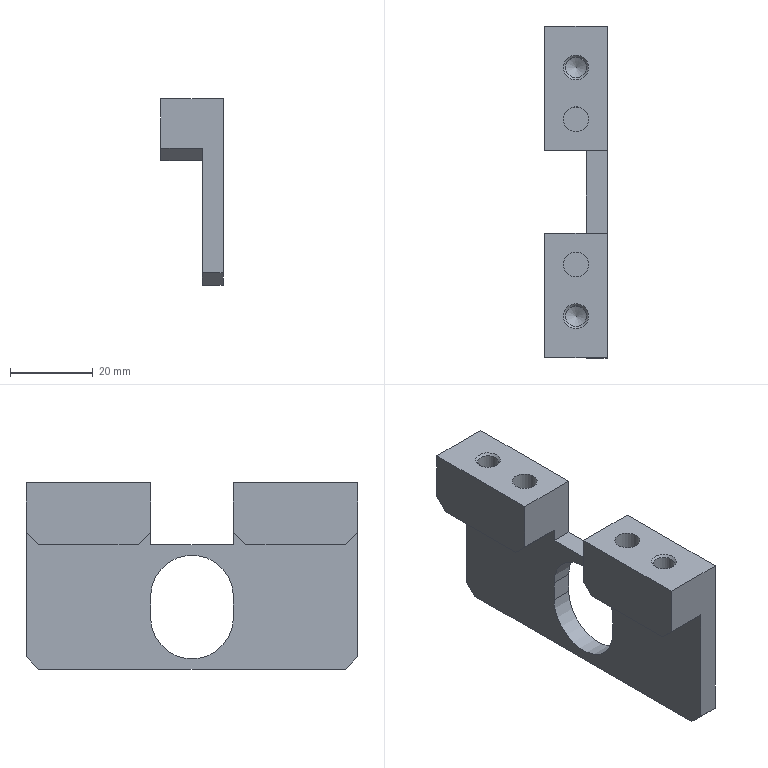Part | STEP file | Tube feed_id822_x_t | 1 solid | 34 faces | box 15 x 80 x 45 mm | volume 22144 mm3 | plane 24 | cylinder 6 | cone 4 | commonest cylinder face diameters 5 x2 6 x2 20 x2